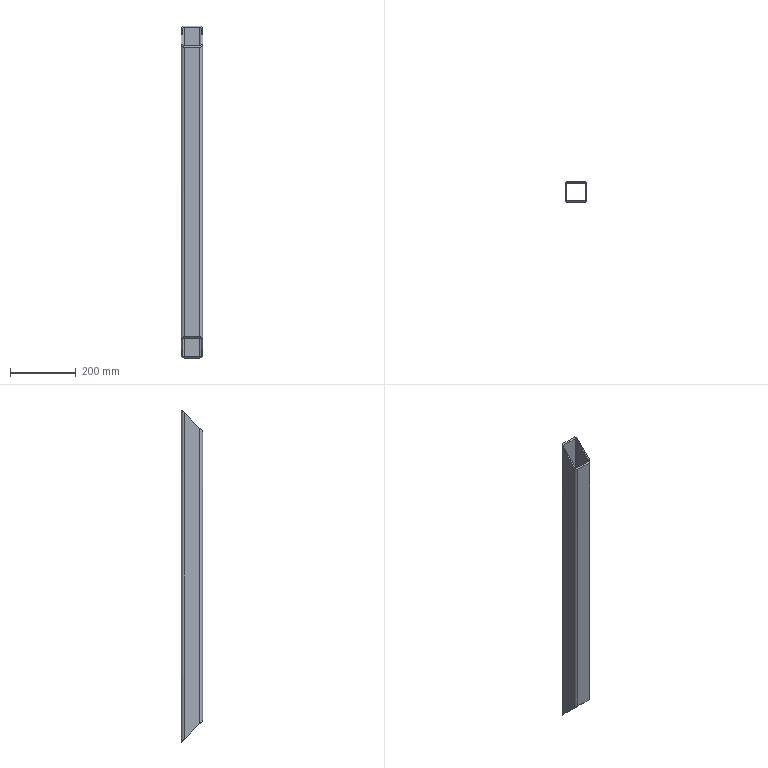Part | SolidWorks | features Extrusion 1, ICE 1 | 1 solid | 18 faces | box 64 x 64 x 1007 mm | volume 866205 mm3 | plane 10 | cylinder 8 | commonest cylinder face diameters 8 x4 16 x4
STEP:
#1=CARTESIAN_POINT('',(-24.,28.,499.38));
#2=VERTEX_POINT('',#1);
#3=CARTESIAN_POINT('',(24.,28.,499.38));
#4=VERTEX_POINT('',#3);
#5=CARTESIAN_POINT('',(0.,28.,499.38));
#6=DIRECTION('',(1.,0.,0.));
#7=VECTOR('',#6,1000.);
#8=LINE('',#5,#7);
#9=EDGE_CURVE('',#2,#4,#8,.T.);
#10=ORIENTED_EDGE('',*,*,#9,.F.);
#11=CARTESIAN_POINT('',(-24.,28.,-499.38));
#12=VERTEX_POINT('',#11);
#13=CARTESIAN_POINT('',(-24.,28.,503.38));
#14=DIRECTION('',(0.,0.,-1.));
#15=VECTOR('',#14,1000.);
#16=LINE('',#13,#15);
#17=EDGE_CURVE('',#2,#12,#16,.T.);
#18=ORIENTED_EDGE('',*,*,#17,.T.);
#19=CARTESIAN_POINT('',(24.,28.,-499.38));
#20=VERTEX_POINT('',#19);
#21=CARTESIAN_POINT('',(0.,28.,-499.38));
#22=DIRECTION('',(-1.,0.,0.));
#23=VECTOR('',#22,1000.);
#24=LINE('',#21,#23);
#25=EDGE_CURVE('',#20,#12,#24,.T.);
#26=ORIENTED_EDGE('',*,*,#25,.F.);
#27=CARTESIAN_POINT('',(24.,28.,503.38));
#28=DIRECTION('',(0.,0.,-1.));
#29=VECTOR('',#28,1000.);
#30=LINE('',#27,#29);
#31=EDGE_CURVE('',#4,#20,#30,.T.);
#32=ORIENTED_EDGE('',*,*,#31,.F.);
#33=EDGE_LOOP('',(#10,#18,#26,#32));
#34=FACE_OUTER_BOUND('',#33,.T.);
#35=CARTESIAN_POINT('',(0.,28.,503.38));
#36=DIRECTION('',(0.,-1.,0.));
#37=DIRECTION('',(0.,0.,-1.));
#38=AXIS2_PLACEMENT_3D('',#35,#36,#37);
#39=PLANE('',#38);
#40=ADVANCED_FACE('',(#34),#39,.T.);
#41=CARTESIAN_POINT('',(28.,24.,495.38));
#42=VERTEX_POINT('',#41);
#43=CARTESIAN_POINT('',(24.,28.,499.38));
#44=CARTESIAN_POINT('',(26.343,28.,499.38));
#45=CARTESIAN_POINT('',(28.,26.343,497.723));
#46=CARTESIAN_POINT('',(28.,24.,495.38));
#47=(BOUNDED_CURVE()B_SPLINE_CURVE(3,(#43,#44,#45,#46),.UNSPECIFIED.,.F.,.T.)B_SPLINE_CURVE_WITH_KNOTS((4,4),(3.142,4.712),.UNSPECIFIED.)CURVE()GEOMETRIC_REPRESENTATION_ITEM()RATIONAL_B_SPLINE_CURVE((1.,0.8047,0.8047,1.))REPRESENTATION_ITEM(''));
#48=EDGE_CURVE('',#4,#42,#47,.T.);
#49=ORIENTED_EDGE('',*,*,#48,.F.);
#50=ORIENTED_EDGE('',*,*,#31,.T.);
#51=CARTESIAN_POINT('',(28.,24.,-495.38));
#52=VERTEX_POINT('',#51);
#53=CARTESIAN_POINT('',(28.,24.,-495.38));
#54=CARTESIAN_POINT('',(28.,26.343,-497.723));
#55=CARTESIAN_POINT('',(26.343,28.,-499.38));
#56=CARTESIAN_POINT('',(24.,28.,-499.38));
#57=(BOUNDED_CURVE()B_SPLINE_CURVE(3,(#53,#54,#55,#56),.UNSPECIFIED.,.F.,.F.)B_SPLINE_CURVE_WITH_KNOTS((4,4),(4.712,6.283),.UNSPECIFIED.)CURVE()GEOMETRIC_REPRESENTATION_ITEM()RATIONAL_B_SPLINE_CURVE((1.,0.8047,0.8047,1.))REPRESENTATION_ITEM(''));
#58=EDGE_CURVE('',#52,#20,#57,.T.);
#59=ORIENTED_EDGE('',*,*,#58,.F.);
#60=CARTESIAN_POINT('',(28.,24.,503.38));
#61=DIRECTION('',(0.,0.,-1.));
#62=VECTOR('',#61,1000.);
#63=LINE('',#60,#62);
#64=EDGE_CURVE('',#42,#52,#63,.T.);
#65=ORIENTED_EDGE('',*,*,#64,.F.);
#66=EDGE_LOOP('',(#49,#50,#59,#65));
#67=FACE_OUTER_BOUND('',#66,.T.);
#68=CARTESIAN_POINT('',(24.,24.,503.38));
#69=DIRECTION('',(0.,0.,-1.));
#70=DIRECTION('',(-1.,0.,0.));
#71=AXIS2_PLACEMENT_3D('',#68,#69,#70);
#72=CYLINDRICAL_SURFACE('',#71,4.);
#73=ADVANCED_FACE('',(#67),#72,.F.);
#74=CARTESIAN_POINT('',(28.,-24.,447.38));
#75=VERTEX_POINT('',#74);
#76=CARTESIAN_POINT('',(28.,28.,499.38));
#77=DIRECTION('',(0.,-0.7071,-0.7071));
#78=VECTOR('',#77,1000.);
#79=LINE('',#76,#78);
#80=EDGE_CURVE('',#42,#75,#79,.T.);
#81=ORIENTED_EDGE('',*,*,#80,.F.);
#82=ORIENTED_EDGE('',*,*,#64,.T.);
#83=CARTESIAN_POINT('',(28.,-24.,-447.38));
#84=VERTEX_POINT('',#83);
#85=CARTESIAN_POINT('',(28.,-475.38,4.));
#86=DIRECTION('',(0.,0.7071,-0.7071));
#87=VECTOR('',#86,1000.);
#88=LINE('',#85,#87);
#89=EDGE_CURVE('',#84,#52,#88,.T.);
#90=ORIENTED_EDGE('',*,*,#89,.F.);
#91=CARTESIAN_POINT('',(28.,-24.,503.38));
#92=DIRECTION('',(0.,0.,-1.));
#93=VECTOR('',#92,1000.);
#94=LINE('',#91,#93);
#95=EDGE_CURVE('',#75,#84,#94,.T.);
#96=ORIENTED_EDGE('',*,*,#95,.F.);
#97=EDGE_LOOP('',(#81,#82,#90,#96));
#98=FACE_OUTER_BOUND('',#97,.T.);
#99=CARTESIAN_POINT('',(28.,24.,503.38));
#100=DIRECTION('',(-1.,0.,0.));
#101=DIRECTION('',(0.,-1.,0.));
#102=AXIS2_PLACEMENT_3D('',#99,#100,#101);
#103=PLANE('',#102);
#104=ADVANCED_FACE('',(#98),#103,.T.);
#105=CARTESIAN_POINT('',(24.,-28.,443.38));
#106=VERTEX_POINT('',#105);
#107=CARTESIAN_POINT('',(28.,-24.,447.38));
#108=CARTESIAN_POINT('',(28.,-26.343,445.037));
#109=CARTESIAN_POINT('',(26.343,-28.,443.38));
#110=CARTESIAN_POINT('',(24.,-28.,443.38));
#111=(BOUNDED_CURVE()B_SPLINE_CURVE(3,(#107,#108,#109,#110),.UNSPECIFIED.,.F.,.F.)B_SPLINE_CURVE_WITH_KNOTS((4,4),(4.712,6.283),.UNSPECIFIED.)CURVE()GEOMETRIC_REPRESENTATION_ITEM()RATIONAL_B_SPLINE_CURVE((1.,0.8047,0.8047,1.))REPRESENTATION_ITEM(''));
#112=EDGE_CURVE('',#75,#106,#111,.T.);
#113=ORIENTED_EDGE('',*,*,#112,.F.);
#114=ORIENTED_EDGE('',*,*,#95,.T.);
#115=CARTESIAN_POINT('',(24.,-28.,-443.38));
#116=VERTEX_POINT('',#115);
#117=CARTESIAN_POINT('',(24.,-28.,-443.38));
#118=CARTESIAN_POINT('',(26.343,-28.,-443.38));
#119=CARTESIAN_POINT('',(28.,-26.343,-445.037));
#120=CARTESIAN_POINT('',(28.,-24.,-447.38));
#121=(BOUNDED_CURVE()B_SPLINE_CURVE(3,(#117,#118,#119,#120),.UNSPECIFIED.,.F.,.F.)B_SPLINE_CURVE_WITH_KNOTS((4,4),(3.142,4.712),.UNSPECIFIED.)CURVE()GEOMETRIC_REPRESENTATION_ITEM()RATIONAL_B_SPLINE_CURVE((1.,0.8047,0.8047,1.))REPRESENTATION_ITEM(''));
#122=EDGE_CURVE('',#116,#84,#121,.T.);
#123=ORIENTED_EDGE('',*,*,#122,.F.);
#124=CARTESIAN_POINT('',(24.,-28.,503.38));
#125=DIRECTION('',(0.,0.,-1.));
#126=VECTOR('',#125,1000.);
#127=LINE('',#124,#126);
#128=EDGE_CURVE('',#106,#116,#127,.T.);
#129=ORIENTED_EDGE('',*,*,#128,.F.);
#130=EDGE_LOOP('',(#113,#114,#123,#129));
#131=FACE_OUTER_BOUND('',#130,.T.);
#132=CARTESIAN_POINT('',(24.,-24.,503.38));
#133=DIRECTION('',(0.,0.,-1.));
#134=DIRECTION('',(-1.,0.,0.));
#135=AXIS2_PLACEMENT_3D('',#132,#133,#134);
#136=CYLINDRICAL_SURFACE('',#135,4.);
#137=ADVANCED_FACE('',(#131),#136,.F.);
#138=CARTESIAN_POINT('',(-24.,-28.,443.38));
#139=VERTEX_POINT('',#138);
#140=CARTESIAN_POINT('',(24.,-28.,443.38));
#141=DIRECTION('',(-1.,0.,0.));
#142=VECTOR('',#141,1000.);
#143=LINE('',#140,#142);
#144=EDGE_CURVE('',#106,#139,#143,.T.);
#145=ORIENTED_EDGE('',*,*,#144,.F.);
#146=ORIENTED_EDGE('',*,*,#128,.T.);
#147=CARTESIAN_POINT('',(-24.,-28.,-443.38));
#148=VERTEX_POINT('',#147);
#149=CARTESIAN_POINT('',(24.,-28.,-443.38));
#150=DIRECTION('',(1.,0.,0.));
#151=VECTOR('',#150,1000.);
#152=LINE('',#149,#151);
#153=EDGE_CURVE('',#148,#116,#152,.T.);
#154=ORIENTED_EDGE('',*,*,#153,.F.);
#155=CARTESIAN_POINT('',(-24.,-28.,503.38));
#156=DIRECTION('',(0.,0.,-1.));
#157=VECTOR('',#156,1000.);
#158=LINE('',#155,#157);
#159=EDGE_CURVE('',#139,#148,#158,.T.);
#160=ORIENTED_EDGE('',*,*,#159,.F.);
#161=EDGE_LOOP('',(#145,#146,#154,#160));
#162=FACE_OUTER_BOUND('',#161,.T.);
#163=CARTESIAN_POINT('',(24.,-28.,503.38));
#164=DIRECTION('',(0.,1.,0.));
#165=DIRECTION('',(-1.,0.,0.));
#166=AXIS2_PLACEMENT_3D('',#163,#164,#165);
#167=PLANE('',#166);
#168=ADVANCED_FACE('',(#162),#167,.T.);
#169=CARTESIAN_POINT('',(-28.,-24.,447.38));
#170=VERTEX_POINT('',#169);
#171=CARTESIAN_POINT('',(-24.,-28.,443.38));
#172=CARTESIAN_POINT('',(-26.343,-28.,443.38));
#173=CARTESIAN_POINT('',(-28.,-26.343,445.037));
#174=CARTESIAN_POINT('',(-28.,-24.,447.38));
#175=(BOUNDED_CURVE()B_SPLINE_CURVE(3,(#171,#172,#173,#174),.UNSPECIFIED.,.F.,.T.)B_SPLINE_CURVE_WITH_KNOTS((4,4),(0.,1.571),.UNSPECIFIED.)CURVE()GEOMETRIC_REPRESENTATION_ITEM()RATIONAL_B_SPLINE_CURVE((1.,0.8047,0.8047,1.))REPRESENTATION_ITEM(''));
#176=EDGE_CURVE('',#139,#170,#175,.T.);
#177=ORIENTED_EDGE('',*,*,#176,.F.);
#178=ORIENTED_EDGE('',*,*,#159,.T.);
#179=CARTESIAN_POINT('',(-28.,-24.,-447.38));
#180=VERTEX_POINT('',#179);
#181=CARTESIAN_POINT('',(-28.,-24.,-447.38));
#182=CARTESIAN_POINT('',(-28.,-26.343,-445.037));
#183=CARTESIAN_POINT('',(-26.343,-28.,-443.38));
#184=CARTESIAN_POINT('',(-24.,-28.,-443.38));
#185=(BOUNDED_CURVE()B_SPLINE_CURVE(3,(#181,#182,#183,#184),.UNSPECIFIED.,.F.,.F.)B_SPLINE_CURVE_WITH_KNOTS((4,4),(1.571,3.142),.UNSPECIFIED.)CURVE()GEOMETRIC_REPRESENTATION_ITEM()RATIONAL_B_SPLINE_CURVE((1.,0.8047,0.8047,1.))REPRESENTATION_ITEM(''));
#186=EDGE_CURVE('',#180,#148,#185,.T.);
#187=ORIENTED_EDGE('',*,*,#186,.F.);
#188=CARTESIAN_POINT('',(-28.,-24.,503.38));
#189=DIRECTION('',(0.,0.,-1.));
#190=VECTOR('',#189,1000.);
#191=LINE('',#188,#190);
#192=EDGE_CURVE('',#170,#180,#191,.T.);
#193=ORIENTED_EDGE('',*,*,#192,.F.);
#194=EDGE_LOOP('',(#177,#178,#187,#193));
#195=FACE_OUTER_BOUND('',#194,.T.);
#196=CARTESIAN_POINT('',(-24.,-24.,503.38));
#197=DIRECTION('',(0.,0.,-1.));
#198=DIRECTION('',(-1.,0.,0.));
#199=AXIS2_PLACEMENT_3D('',#196,#197,#198);
#200=CYLINDRICAL_SURFACE('',#199,4.);
#201=ADVANCED_FACE('',(#195),#200,.F.);
#202=CARTESIAN_POINT('',(-28.,24.,495.38));
#203=VERTEX_POINT('',#202);
#204=CARTESIAN_POINT('',(-28.,4.,475.38));
#205=DIRECTION('',(0.,0.7071,0.7071));
#206=VECTOR('',#205,1000.);
#207=LINE('',#204,#206);
#208=EDGE_CURVE('',#170,#203,#207,.T.);
#209=ORIENTED_EDGE('',*,*,#208,.F.);
#210=ORIENTED_EDGE('',*,*,#192,.T.);
#211=CARTESIAN_POINT('',(-28.,24.,-495.38));
#212=VERTEX_POINT('',#211);
#213=CARTESIAN_POINT('',(-28.,-499.38,28.));
#214=DIRECTION('',(0.,-0.7071,0.7071));
#215=VECTOR('',#214,1000.);
#216=LINE('',#213,#215);
#217=EDGE_CURVE('',#212,#180,#216,.T.);
#218=ORIENTED_EDGE('',*,*,#217,.F.);
#219=CARTESIAN_POINT('',(-28.,24.,503.38));
#220=DIRECTION('',(0.,0.,-1.));
#221=VECTOR('',#220,1000.);
#222=LINE('',#219,#221);
#223=EDGE_CURVE('',#203,#212,#222,.T.);
#224=ORIENTED_EDGE('',*,*,#223,.F.);
#225=EDGE_LOOP('',(#209,#210,#218,#224));
#226=FACE_OUTER_BOUND('',#225,.T.);
#227=CARTESIAN_POINT('',(-28.,-24.,503.38));
#228=DIRECTION('',(1.,0.,0.));
#229=DIRECTION('',(0.,1.,0.));
#230=AXIS2_PLACEMENT_3D('',#227,#228,#229);
#231=PLANE('',#230);
#232=ADVANCED_FACE('',(#226),#231,.T.);
#233=CARTESIAN_POINT('',(-28.,24.,495.38));
#234=CARTESIAN_POINT('',(-28.,26.343,497.723));
#235=CARTESIAN_POINT('',(-26.343,28.,499.38));
#236=CARTESIAN_POINT('',(-24.,28.,499.38));
#237=(BOUNDED_CURVE()B_SPLINE_CURVE(3,(#233,#234,#235,#236),.UNSPECIFIED.,.F.,.T.)B_SPLINE_CURVE_WITH_KNOTS((4,4),(1.571,3.142),.UNSPECIFIED.)CURVE()GEOMETRIC_REPRESENTATION_ITEM()RATIONAL_B_SPLINE_CURVE((1.,0.8047,0.8047,1.))REPRESENTATION_ITEM(''));
#238=EDGE_CURVE('',#203,#2,#237,.T.);
#239=ORIENTED_EDGE('',*,*,#238,.F.);
#240=ORIENTED_EDGE('',*,*,#223,.T.);
#241=CARTESIAN_POINT('',(-24.,28.,-499.38));
#242=CARTESIAN_POINT('',(-26.343,28.,-499.38));
#243=CARTESIAN_POINT('',(-28.,26.343,-497.723));
#244=CARTESIAN_POINT('',(-28.,24.,-495.38));
#245=(BOUNDED_CURVE()B_SPLINE_CURVE(3,(#241,#242,#243,#244),.UNSPECIFIED.,.F.,.F.)B_SPLINE_CURVE_WITH_KNOTS((4,4),(0.,1.571),.UNSPECIFIED.)CURVE()GEOMETRIC_REPRESENTATION_ITEM()RATIONAL_B_SPLINE_CURVE((1.,0.8047,0.8047,1.))REPRESENTATION_ITEM(''));
#246=EDGE_CURVE('',#12,#212,#245,.T.);
#247=ORIENTED_EDGE('',*,*,#246,.F.);
#248=ORIENTED_EDGE('',*,*,#17,.F.);
#249=EDGE_LOOP('',(#239,#240,#247,#248));
#250=FACE_OUTER_BOUND('',#249,.T.);
#251=CARTESIAN_POINT('',(-24.,24.,503.38));
#252=DIRECTION('',(0.,0.,-1.));
#253=DIRECTION('',(-1.,0.,0.));
#254=AXIS2_PLACEMENT_3D('',#251,#252,#253);
#255=CYLINDRICAL_SURFACE('',#254,4.);
#256=ADVANCED_FACE('',(#250),#255,.F.);
#257=ORIENTED_EDGE('',*,*,#246,.T.);
#258=ORIENTED_EDGE('',*,*,#217,.T.);
#259=ORIENTED_EDGE('',*,*,#186,.T.);
#260=ORIENTED_EDGE('',*,*,#153,.T.);
#261=ORIENTED_EDGE('',*,*,#122,.T.);
#262=ORIENTED_EDGE('',*,*,#89,.T.);
#263=ORIENTED_EDGE('',*,*,#58,.T.);
#264=ORIENTED_EDGE('',*,*,#25,.T.);
#265=EDGE_LOOP('',(#257,#258,#259,#260,#261,#262,#263,#264));
#266=FACE_BOUND('',#265,.T.);
#267=CARTESIAN_POINT('',(24.,32.,-503.38));
#268=VERTEX_POINT('',#267);
#269=CARTESIAN_POINT('',(-24.,32.,-503.38));
#270=VERTEX_POINT('',#269);
#271=CARTESIAN_POINT('',(0.,32.,-503.38));
#272=DIRECTION('',(-1.,0.,0.));
#273=VECTOR('',#272,1000.);
#274=LINE('',#271,#273);
#275=EDGE_CURVE('',#268,#270,#274,.T.);
#276=ORIENTED_EDGE('',*,*,#275,.F.);
#277=CARTESIAN_POINT('',(32.,24.,-495.38));
#278=VERTEX_POINT('',#277);
#279=CARTESIAN_POINT('',(32.,24.,-495.38));
#280=CARTESIAN_POINT('',(32.,28.686,-500.066));
#281=CARTESIAN_POINT('',(28.686,32.,-503.38));
#282=CARTESIAN_POINT('',(24.,32.,-503.38));
#283=(BOUNDED_CURVE()B_SPLINE_CURVE(3,(#279,#280,#281,#282),.UNSPECIFIED.,.F.,.T.)B_SPLINE_CURVE_WITH_KNOTS((4,4),(4.712,6.283),.UNSPECIFIED.)CURVE()GEOMETRIC_REPRESENTATION_ITEM()RATIONAL_B_SPLINE_CURVE((1.,0.8047,0.8047,1.))REPRESENTATION_ITEM(''));
#284=EDGE_CURVE('',#278,#268,#283,.T.);
#285=ORIENTED_EDGE('',*,*,#284,.F.);
#286=CARTESIAN_POINT('',(32.,-24.,-447.38));
#287=VERTEX_POINT('',#286);
#288=CARTESIAN_POINT('',(32.,32.,-503.38));
#289=DIRECTION('',(0.,-0.7071,0.7071));
#290=VECTOR('',#289,1000.);
#291=LINE('',#288,#290);
#292=EDGE_CURVE('',#278,#287,#291,.T.);
#293=ORIENTED_EDGE('',*,*,#292,.T.);
#294=CARTESIAN_POINT('',(24.,-32.,-439.38));
#295=VERTEX_POINT('',#294);
#296=CARTESIAN_POINT('',(24.,-32.,-439.38));
#297=CARTESIAN_POINT('',(28.686,-32.,-439.38));
#298=CARTESIAN_POINT('',(32.,-28.686,-442.694));
#299=CARTESIAN_POINT('',(32.,-24.,-447.38));
#300=(BOUNDED_CURVE()B_SPLINE_CURVE(3,(#296,#297,#298,#299),.UNSPECIFIED.,.F.,.F.)B_SPLINE_CURVE_WITH_KNOTS((4,4),(3.142,4.712),.UNSPECIFIED.)CURVE()GEOMETRIC_REPRESENTATION_ITEM()RATIONAL_B_SPLINE_CURVE((1.,0.8047,0.8047,1.))REPRESENTATION_ITEM(''));
#301=EDGE_CURVE('',#295,#287,#300,.T.);
#302=ORIENTED_EDGE('',*,*,#301,.F.);
#303=CARTESIAN_POINT('',(-24.,-32.,-439.38));
#304=VERTEX_POINT('',#303);
#305=CARTESIAN_POINT('',(-32.,-32.,-439.38));
#306=DIRECTION('',(1.,0.,0.));
#307=VECTOR('',#306,1000.);
#308=LINE('',#305,#307);
#309=EDGE_CURVE('',#304,#295,#308,.T.);
#310=ORIENTED_EDGE('',*,*,#309,.F.);
#311=CARTESIAN_POINT('',(-32.,-24.,-447.38));
#312=VERTEX_POINT('',#311);
#313=CARTESIAN_POINT('',(-32.,-24.,-447.38));
#314=CARTESIAN_POINT('',(-32.,-28.686,-442.694));
#315=CARTESIAN_POINT('',(-28.686,-32.,-439.38));
#316=CARTESIAN_POINT('',(-24.,-32.,-439.38));
#317=(BOUNDED_CURVE()B_SPLINE_CURVE(3,(#313,#314,#315,#316),.UNSPECIFIED.,.F.,.T.)B_SPLINE_CURVE_WITH_KNOTS((4,4),(1.571,3.142),.UNSPECIFIED.)CURVE()GEOMETRIC_REPRESENTATION_ITEM()RATIONAL_B_SPLINE_CURVE((1.,0.8047,0.8047,1.))REPRESENTATION_ITEM(''));
#318=EDGE_CURVE('',#312,#304,#317,.T.);
#319=ORIENTED_EDGE('',*,*,#318,.F.);
#320=CARTESIAN_POINT('',(-32.,24.,-495.38));
#321=VERTEX_POINT('',#320);
#322=CARTESIAN_POINT('',(-32.,32.,-503.38));
#323=DIRECTION('',(0.,-0.7071,0.7071));
#324=VECTOR('',#323,1000.);
#325=LINE('',#322,#324);
#326=EDGE_CURVE('',#321,#312,#325,.T.);
#327=ORIENTED_EDGE('',*,*,#326,.F.);
#328=CARTESIAN_POINT('',(-24.,32.,-503.38));
#329=CARTESIAN_POINT('',(-28.686,32.,-503.38));
#330=CARTESIAN_POINT('',(-32.,28.686,-500.066));
#331=CARTESIAN_POINT('',(-32.,24.,-495.38));
#332=(BOUNDED_CURVE()B_SPLINE_CURVE(3,(#328,#329,#330,#331),.UNSPECIFIED.,.F.,.T.)B_SPLINE_CURVE_WITH_KNOTS((4,4),(0.,1.571),.UNSPECIFIED.)CURVE()GEOMETRIC_REPRESENTATION_ITEM()RATIONAL_B_SPLINE_CURVE((1.,0.8047,0.8047,1.))REPRESENTATION_ITEM(''));
#333=EDGE_CURVE('',#270,#321,#332,.T.);
#334=ORIENTED_EDGE('',*,*,#333,.F.);
#335=EDGE_LOOP('',(#276,#285,#293,#302,#310,#319,#327,#334));
#336=FACE_OUTER_BOUND('',#335,.T.);
#337=CARTESIAN_POINT('',(-32.,32.,-503.38));
#338=DIRECTION('',(0.,0.7071,0.7071));
#339=DIRECTION('',(0.,-0.7071,0.7071));
#340=AXIS2_PLACEMENT_3D('',#337,#338,#339);
#341=PLANE('',#340);
#342=ADVANCED_FACE('',(#266,#336),#341,.F.);
#343=ORIENTED_EDGE('',*,*,#238,.T.);
#344=ORIENTED_EDGE('',*,*,#9,.T.);
#345=ORIENTED_EDGE('',*,*,#48,.T.);
#346=ORIENTED_EDGE('',*,*,#80,.T.);
#347=ORIENTED_EDGE('',*,*,#112,.T.);
#348=ORIENTED_EDGE('',*,*,#144,.T.);
#349=ORIENTED_EDGE('',*,*,#176,.T.);
#350=ORIENTED_EDGE('',*,*,#208,.T.);
#351=EDGE_LOOP('',(#343,#344,#345,#346,#347,#348,#349,#350));
#352=FACE_BOUND('',#351,.T.);
#353=CARTESIAN_POINT('',(-32.,-24.,447.38));
#354=VERTEX_POINT('',#353);
#355=CARTESIAN_POINT('',(-32.,24.,495.38));
#356=VERTEX_POINT('',#355);
#357=CARTESIAN_POINT('',(-32.,32.,503.38));
#358=DIRECTION('',(0.,0.7071,0.7071));
#359=VECTOR('',#358,1000.);
#360=LINE('',#357,#359);
#361=EDGE_CURVE('',#354,#356,#360,.T.);
#362=ORIENTED_EDGE('',*,*,#361,.F.);
#363=CARTESIAN_POINT('',(-24.,-32.,439.38));
#364=VERTEX_POINT('',#363);
#365=CARTESIAN_POINT('',(-24.,-32.,439.38));
#366=CARTESIAN_POINT('',(-28.686,-32.,439.38));
#367=CARTESIAN_POINT('',(-32.,-28.686,442.694));
#368=CARTESIAN_POINT('',(-32.,-24.,447.38));
#369=(BOUNDED_CURVE()B_SPLINE_CURVE(3,(#365,#366,#367,#368),.UNSPECIFIED.,.F.,.F.)B_SPLINE_CURVE_WITH_KNOTS((4,4),(0.,1.571),.UNSPECIFIED.)CURVE()GEOMETRIC_REPRESENTATION_ITEM()RATIONAL_B_SPLINE_CURVE((1.,0.8047,0.8047,1.))REPRESENTATION_ITEM(''));
#370=EDGE_CURVE('',#364,#354,#369,.T.);
#371=ORIENTED_EDGE('',*,*,#370,.F.);
#372=CARTESIAN_POINT('',(24.,-32.,439.38));
#373=VERTEX_POINT('',#372);
#374=CARTESIAN_POINT('',(-32.,-32.,439.38));
#375=DIRECTION('',(1.,0.,0.));
#376=VECTOR('',#375,1000.);
#377=LINE('',#374,#376);
#378=EDGE_CURVE('',#364,#373,#377,.T.);
#379=ORIENTED_EDGE('',*,*,#378,.T.);
#380=CARTESIAN_POINT('',(32.,-24.,447.38));
#381=VERTEX_POINT('',#380);
#382=CARTESIAN_POINT('',(32.,-24.,447.38));
#383=CARTESIAN_POINT('',(32.,-28.686,442.694));
#384=CARTESIAN_POINT('',(28.686,-32.,439.38));
#385=CARTESIAN_POINT('',(24.,-32.,439.38));
#386=(BOUNDED_CURVE()B_SPLINE_CURVE(3,(#382,#383,#384,#385),.UNSPECIFIED.,.F.,.T.)B_SPLINE_CURVE_WITH_KNOTS((4,4),(4.712,6.283),.UNSPECIFIED.)CURVE()GEOMETRIC_REPRESENTATION_ITEM()RATIONAL_B_SPLINE_CURVE((1.,0.8047,0.8047,1.))REPRESENTATION_ITEM(''));
#387=EDGE_CURVE('',#381,#373,#386,.T.);
#388=ORIENTED_EDGE('',*,*,#387,.F.);
#389=CARTESIAN_POINT('',(32.,24.,495.38));
#390=VERTEX_POINT('',#389);
#391=CARTESIAN_POINT('',(32.,32.,503.38));
#392=DIRECTION('',(0.,0.7071,0.7071));
#393=VECTOR('',#392,1000.);
#394=LINE('',#391,#393);
#395=EDGE_CURVE('',#381,#390,#394,.T.);
#396=ORIENTED_EDGE('',*,*,#395,.T.);
#397=CARTESIAN_POINT('',(24.,32.,503.38));
#398=VERTEX_POINT('',#397);
#399=CARTESIAN_POINT('',(24.,32.,503.38));
#400=CARTESIAN_POINT('',(28.686,32.,503.38));
#401=CARTESIAN_POINT('',(32.,28.686,500.066));
#402=CARTESIAN_POINT('',(32.,24.,495.38));
#403=(BOUNDED_CURVE()B_SPLINE_CURVE(3,(#399,#400,#401,#402),.UNSPECIFIED.,.F.,.F.)B_SPLINE_CURVE_WITH_KNOTS((4,4),(3.142,4.712),.UNSPECIFIED.)CURVE()GEOMETRIC_REPRESENTATION_ITEM()RATIONAL_B_SPLINE_CURVE((1.,0.8047,0.8047,1.))REPRESENTATION_ITEM(''));
#404=EDGE_CURVE('',#398,#390,#403,.T.);
#405=ORIENTED_EDGE('',*,*,#404,.F.);
#406=CARTESIAN_POINT('',(-24.,32.,503.38));
#407=VERTEX_POINT('',#406);
#408=CARTESIAN_POINT('',(0.,32.,503.38));
#409=DIRECTION('',(-1.,0.,0.));
#410=VECTOR('',#409,1000.);
#411=LINE('',#408,#410);
#412=EDGE_CURVE('',#398,#407,#411,.T.);
#413=ORIENTED_EDGE('',*,*,#412,.T.);
#414=CARTESIAN_POINT('',(-32.,24.,495.38));
#415=CARTESIAN_POINT('',(-32.,28.686,500.066));
#416=CARTESIAN_POINT('',(-28.686,32.,503.38));
#417=CARTESIAN_POINT('',(-24.,32.,503.38));
#418=(BOUNDED_CURVE()B_SPLINE_CURVE(3,(#414,#415,#416,#417),.UNSPECIFIED.,.F.,.F.)B_SPLINE_CURVE_WITH_KNOTS((4,4),(1.571,3.142),.UNSPECIFIED.)CURVE()GEOMETRIC_REPRESENTATION_ITEM()RATIONAL_B_SPLINE_CURVE((1.,0.8047,0.8047,1.))REPRESENTATION_ITEM(''));
#419=EDGE_CURVE('',#356,#407,#418,.T.);
#420=ORIENTED_EDGE('',*,*,#419,.F.);
#421=EDGE_LOOP('',(#362,#371,#379,#388,#396,#405,#413,#420));
#422=FACE_OUTER_BOUND('',#421,.T.);
#423=CARTESIAN_POINT('',(-32.,32.,503.38));
#424=DIRECTION('',(0.,0.7071,-0.7071));
#425=DIRECTION('',(0.,0.7071,0.7071));
#426=AXIS2_PLACEMENT_3D('',#423,#424,#425);
#427=PLANE('',#426);
#428=ADVANCED_FACE('',(#352,#422),#427,.F.);
#429=CARTESIAN_POINT('',(-32.,24.,503.38));
#430=DIRECTION('',(0.,0.,-1.));
#431=VECTOR('',#430,1000.);
#432=LINE('',#429,#431);
#433=EDGE_CURVE('',#356,#321,#432,.T.);
#434=ORIENTED_EDGE('',*,*,#433,.F.);
#435=ORIENTED_EDGE('',*,*,#419,.T.);
#436=CARTESIAN_POINT('',(-24.,32.,503.38));
#437=DIRECTION('',(0.,0.,-1.));
#438=VECTOR('',#437,1000.);
#439=LINE('',#436,#438);
#440=EDGE_CURVE('',#407,#270,#439,.T.);
#441=ORIENTED_EDGE('',*,*,#440,.T.);
#442=ORIENTED_EDGE('',*,*,#333,.T.);
#443=EDGE_LOOP('',(#434,#435,#441,#442));
#444=FACE_OUTER_BOUND('',#443,.T.);
#445=CARTESIAN_POINT('',(-24.,24.,503.38));
#446=DIRECTION('',(0.,0.,-1.));
#447=DIRECTION('',(-1.,0.,0.));
#448=AXIS2_PLACEMENT_3D('',#445,#446,#447);
#449=CYLINDRICAL_SURFACE('',#448,8.);
#450=ADVANCED_FACE('',(#444),#449,.T.);
#451=CARTESIAN_POINT('',(-32.,-24.,503.38));
#452=DIRECTION('',(0.,0.,-1.));
#453=VECTOR('',#452,1000.);
#454=LINE('',#451,#453);
#455=EDGE_CURVE('',#354,#312,#454,.T.);
#456=ORIENTED_EDGE('',*,*,#455,.F.);
#457=ORIENTED_EDGE('',*,*,#361,.T.);
#458=ORIENTED_EDGE('',*,*,#433,.T.);
#459=ORIENTED_EDGE('',*,*,#326,.T.);
#460=EDGE_LOOP('',(#456,#457,#458,#459));
#461=FACE_OUTER_BOUND('',#460,.T.);
#462=CARTESIAN_POINT('',(-32.,-24.,503.38));
#463=DIRECTION('',(1.,0.,0.));
#464=DIRECTION('',(0.,0.,-1.));
#465=AXIS2_PLACEMENT_3D('',#462,#463,#464);
#466=PLANE('',#465);
#467=ADVANCED_FACE('',(#461),#466,.F.);
#468=CARTESIAN_POINT('',(-24.,-32.,503.38));
#469=DIRECTION('',(0.,0.,-1.));
#470=VECTOR('',#469,1000.);
#471=LINE('',#468,#470);
#472=EDGE_CURVE('',#364,#304,#471,.T.);
#473=ORIENTED_EDGE('',*,*,#472,.F.);
#474=ORIENTED_EDGE('',*,*,#370,.T.);
#475=ORIENTED_EDGE('',*,*,#455,.T.);
#476=ORIENTED_EDGE('',*,*,#318,.T.);
#477=EDGE_LOOP('',(#473,#474,#475,#476));
#478=FACE_OUTER_BOUND('',#477,.T.);
#479=CARTESIAN_POINT('',(-24.,-24.,503.38));
#480=DIRECTION('',(0.,0.,-1.));
#481=DIRECTION('',(-1.,0.,0.));
#482=AXIS2_PLACEMENT_3D('',#479,#480,#481);
#483=CYLINDRICAL_SURFACE('',#482,8.);
#484=ADVANCED_FACE('',(#478),#483,.T.);
#485=CARTESIAN_POINT('',(24.,-32.,503.38));
#486=DIRECTION('',(0.,0.,-1.));
#487=VECTOR('',#486,1000.);
#488=LINE('',#485,#487);
#489=EDGE_CURVE('',#373,#295,#488,.T.);
#490=ORIENTED_EDGE('',*,*,#489,.F.);
#491=ORIENTED_EDGE('',*,*,#378,.F.);
#492=ORIENTED_EDGE('',*,*,#472,.T.);
#493=ORIENTED_EDGE('',*,*,#309,.T.);
#494=EDGE_LOOP('',(#490,#491,#492,#493));
#495=FACE_OUTER_BOUND('',#494,.T.);
#496=CARTESIAN_POINT('',(24.,-32.,503.38));
#497=DIRECTION('',(0.,1.,0.));
#498=DIRECTION('',(-1.,0.,0.));
#499=AXIS2_PLACEMENT_3D('',#496,#497,#498);
#500=PLANE('',#499);
#501=ADVANCED_FACE('',(#495),#500,.F.);
#502=CARTESIAN_POINT('',(32.,-24.,503.38));
#503=DIRECTION('',(0.,0.,-1.));
#504=VECTOR('',#503,1000.);
#505=LINE('',#502,#504);
#506=EDGE_CURVE('',#381,#287,#505,.T.);
#507=ORIENTED_EDGE('',*,*,#506,.F.);
#508=ORIENTED_EDGE('',*,*,#387,.T.);
#509=ORIENTED_EDGE('',*,*,#489,.T.);
#510=ORIENTED_EDGE('',*,*,#301,.T.);
#511=EDGE_LOOP('',(#507,#508,#509,#510));
#512=FACE_OUTER_BOUND('',#511,.T.);
#513=CARTESIAN_POINT('',(24.,-24.,503.38));
#514=DIRECTION('',(0.,0.,-1.));
#515=DIRECTION('',(-1.,0.,0.));
#516=AXIS2_PLACEMENT_3D('',#513,#514,#515);
#517=CYLINDRICAL_SURFACE('',#516,8.);
#518=ADVANCED_FACE('',(#512),#517,.T.);
#519=CARTESIAN_POINT('',(32.,24.,503.38));
#520=DIRECTION('',(0.,0.,-1.));
#521=VECTOR('',#520,1000.);
#522=LINE('',#519,#521);
#523=EDGE_CURVE('',#390,#278,#522,.T.);
#524=ORIENTED_EDGE('',*,*,#523,.F.);
#525=ORIENTED_EDGE('',*,*,#395,.F.);
#526=ORIENTED_EDGE('',*,*,#506,.T.);
#527=ORIENTED_EDGE('',*,*,#292,.F.);
#528=EDGE_LOOP('',(#524,#525,#526,#527));
#529=FACE_OUTER_BOUND('',#528,.T.);
#530=CARTESIAN_POINT('',(32.,24.,503.38));
#531=DIRECTION('',(-1.,0.,0.));
#532=DIRECTION('',(0.,0.,1.));
#533=AXIS2_PLACEMENT_3D('',#530,#531,#532);
#534=PLANE('',#533);
#535=ADVANCED_FACE('',(#529),#534,.F.);
#536=CARTESIAN_POINT('',(24.,32.,503.38));
#537=DIRECTION('',(0.,0.,-1.));
#538=VECTOR('',#537,1000.);
#539=LINE('',#536,#538);
#540=EDGE_CURVE('',#398,#268,#539,.T.);
#541=ORIENTED_EDGE('',*,*,#540,.F.);
#542=ORIENTED_EDGE('',*,*,#404,.T.);
#543=ORIENTED_EDGE('',*,*,#523,.T.);
#544=ORIENTED_EDGE('',*,*,#284,.T.);
#545=EDGE_LOOP('',(#541,#542,#543,#544));
#546=FACE_OUTER_BOUND('',#545,.T.);
#547=CARTESIAN_POINT('',(24.,24.,503.38));
#548=DIRECTION('',(0.,0.,-1.));
#549=DIRECTION('',(-1.,0.,0.));
#550=AXIS2_PLACEMENT_3D('',#547,#548,#549);
#551=CYLINDRICAL_SURFACE('',#550,8.);
#552=ADVANCED_FACE('',(#546),#551,.T.);
#553=ORIENTED_EDGE('',*,*,#275,.T.);
#554=ORIENTED_EDGE('',*,*,#440,.F.);
#555=ORIENTED_EDGE('',*,*,#412,.F.);
#556=ORIENTED_EDGE('',*,*,#540,.T.);
#557=EDGE_LOOP('',(#553,#554,#555,#556));
#558=FACE_OUTER_BOUND('',#557,.T.);
#559=CARTESIAN_POINT('',(0.,32.,503.38));
#560=DIRECTION('',(0.,-1.,0.));
#561=DIRECTION('',(0.,0.,-1.));
#562=AXIS2_PLACEMENT_3D('',#559,#560,#561);
#563=PLANE('',#562);
#564=ADVANCED_FACE('',(#558),#563,.F.);
#565=CLOSED_SHELL('',(#40,#73,#104,#137,#168,#201,#232,#256,#342,#428,#450,#467,#484,#501,#518,#535,#552,#564));
#566=MANIFOLD_SOLID_BREP('',#565);
#567=CARTESIAN_POINT('',(0.,0.,0.));
#568=DIRECTION('',(0.,0.,1.));
#569=DIRECTION('',(1.,0.,0.));
#570=AXIS2_PLACEMENT_3D('',#567,#568,#569);
#571=(LENGTH_UNIT()NAMED_UNIT(*)SI_UNIT(.MILLI.,.METRE.));
#572=UNCERTAINTY_MEASURE_WITH_UNIT(LENGTH_MEASURE(0.00001),#571,'','');
#573=(NAMED_UNIT(*)PLANE_ANGLE_UNIT()SI_UNIT($,.RADIAN.));
#574=(NAMED_UNIT(*)SI_UNIT($,.STERADIAN.)SOLID_ANGLE_UNIT());
#575=(GEOMETRIC_REPRESENTATION_CONTEXT(3)GLOBAL_UNCERTAINTY_ASSIGNED_CONTEXT((#572))GLOBAL_UNIT_ASSIGNED_CONTEXT((#571,#573,#574))REPRESENTATION_CONTEXT('',''));
#576=ADVANCED_BREP_SHAPE_REPRESENTATION('',(#566,#570),#575);